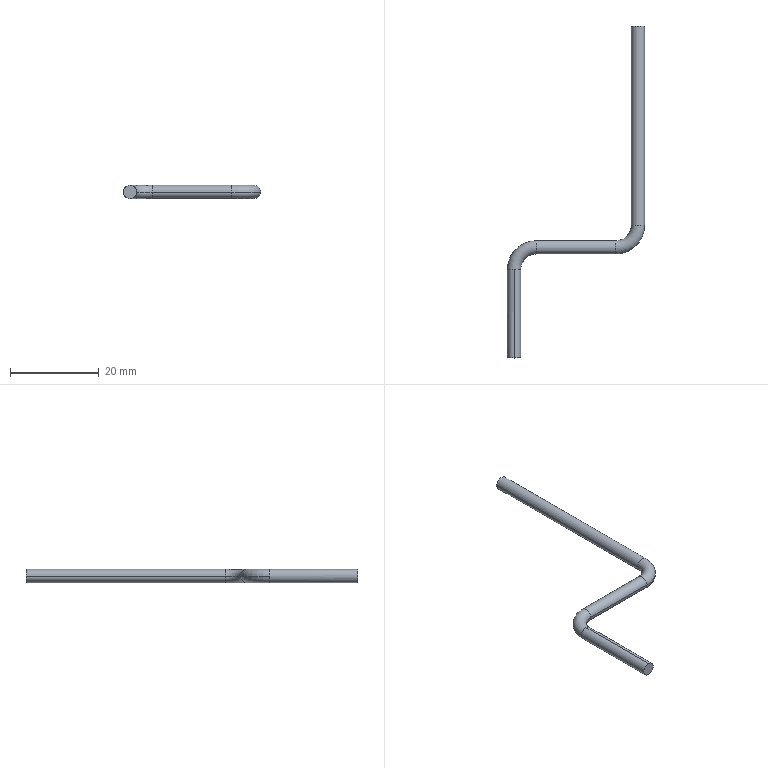Part | SolidWorks | features BaseBody 1 | 1 solid | 12 faces | box 31 x 75 x 3 mm | volume 697.725 mm3 | cylinder 6 | torus 4 | plane 2 | commonest cylinder face diameters 3 x6
STEP:
#1=CARTESIAN_POINT('',(23.,23.5,0.));
#2=VERTEX_POINT('',#1);
#3=CARTESIAN_POINT('',(23.,26.5,0.));
#4=VERTEX_POINT('',#3);
#5=CARTESIAN_POINT('',(23.,25.,0.));
#6=DIRECTION('',(-1.,0.,0.));
#7=DIRECTION('',(0.,0.,-1.));
#8=AXIS2_PLACEMENT_3D('',#5,#6,#7);
#9=CIRCLE('',#8,1.5);
#10=EDGE_CURVE('',#2,#4,#9,.T.);
#11=ORIENTED_EDGE('',*,*,#10,.F.);
#12=CARTESIAN_POINT('',(29.5,30.,0.));
#13=VERTEX_POINT('',#12);
#14=CARTESIAN_POINT('',(23.,30.,0.));
#15=DIRECTION('',(0.,0.,1.));
#16=DIRECTION('',(1.,0.,0.));
#17=AXIS2_PLACEMENT_3D('',#14,#15,#16);
#18=CIRCLE('',#17,6.5);
#19=EDGE_CURVE('',#2,#13,#18,.T.);
#20=ORIENTED_EDGE('',*,*,#19,.T.);
#21=CARTESIAN_POINT('',(26.5,30.,0.));
#22=VERTEX_POINT('',#21);
#23=CARTESIAN_POINT('',(28.,30.,0.));
#24=DIRECTION('',(0.,-1.,0.));
#25=DIRECTION('',(0.,0.,-1.));
#26=AXIS2_PLACEMENT_3D('',#23,#24,#25);
#27=CIRCLE('',#26,1.5);
#28=EDGE_CURVE('',#13,#22,#27,.T.);
#29=ORIENTED_EDGE('',*,*,#28,.T.);
#30=CARTESIAN_POINT('',(23.,30.,0.));
#31=DIRECTION('',(0.,0.,1.));
#32=DIRECTION('',(1.,0.,0.));
#33=AXIS2_PLACEMENT_3D('',#30,#31,#32);
#34=CIRCLE('',#33,3.5);
#35=EDGE_CURVE('',#4,#22,#34,.T.);
#36=ORIENTED_EDGE('',*,*,#35,.F.);
#37=EDGE_LOOP('',(#11,#20,#29,#36));
#38=FACE_OUTER_BOUND('',#37,.T.);
#39=CARTESIAN_POINT('',(23.,30.,0.));
#40=DIRECTION('',(0.,0.,1.));
#41=DIRECTION('',(1.,0.,0.));
#42=AXIS2_PLACEMENT_3D('',#39,#40,#41);
#43=TOROIDAL_SURFACE('',#42,5.,1.5);
#44=ADVANCED_FACE('',(#38),#43,.T.);
#45=CARTESIAN_POINT('',(-1.5,20.,0.));
#46=VERTEX_POINT('',#45);
#47=CARTESIAN_POINT('',(0.,20.,-1.5));
#48=VERTEX_POINT('',#47);
#49=CARTESIAN_POINT('',(0.,20.,0.));
#50=DIRECTION('',(0.,-1.,0.));
#51=DIRECTION('',(0.,0.,-1.));
#52=AXIS2_PLACEMENT_3D('',#49,#50,#51);
#53=CIRCLE('',#52,1.5);
#54=EDGE_CURVE('',#46,#48,#53,.T.);
#55=ORIENTED_EDGE('',*,*,#54,.F.);
#56=CARTESIAN_POINT('',(5.,26.5,0.));
#57=VERTEX_POINT('',#56);
#58=CARTESIAN_POINT('',(5.,20.,0.));
#59=DIRECTION('',(0.,0.,-1.));
#60=DIRECTION('',(-1.,0.,0.));
#61=AXIS2_PLACEMENT_3D('',#58,#59,#60);
#62=CIRCLE('',#61,6.5);
#63=EDGE_CURVE('',#46,#57,#62,.T.);
#64=ORIENTED_EDGE('',*,*,#63,.T.);
#65=CARTESIAN_POINT('',(5.,23.5,0.));
#66=VERTEX_POINT('',#65);
#67=CARTESIAN_POINT('',(5.,25.,0.));
#68=DIRECTION('',(-1.,0.,0.));
#69=DIRECTION('',(0.,0.,-1.));
#70=AXIS2_PLACEMENT_3D('',#67,#68,#69);
#71=CIRCLE('',#70,1.5);
#72=EDGE_CURVE('',#57,#66,#71,.T.);
#73=ORIENTED_EDGE('',*,*,#72,.T.);
#74=CARTESIAN_POINT('',(1.5,20.,0.));
#75=VERTEX_POINT('',#74);
#76=CARTESIAN_POINT('',(5.,20.,0.));
#77=DIRECTION('',(0.,0.,-1.));
#78=DIRECTION('',(-1.,0.,0.));
#79=AXIS2_PLACEMENT_3D('',#76,#77,#78);
#80=CIRCLE('',#79,3.5);
#81=EDGE_CURVE('',#75,#66,#80,.T.);
#82=ORIENTED_EDGE('',*,*,#81,.F.);
#83=CARTESIAN_POINT('',(0.,20.,0.));
#84=DIRECTION('',(0.,-1.,0.));
#85=DIRECTION('',(0.,0.,-1.));
#86=AXIS2_PLACEMENT_3D('',#83,#84,#85);
#87=CIRCLE('',#86,1.5);
#88=EDGE_CURVE('',#48,#75,#87,.T.);
#89=ORIENTED_EDGE('',*,*,#88,.F.);
#90=EDGE_LOOP('',(#55,#64,#73,#82,#89));
#91=FACE_OUTER_BOUND('',#90,.T.);
#92=CARTESIAN_POINT('',(5.,20.,0.));
#93=DIRECTION('',(0.,0.,-1.));
#94=DIRECTION('',(-1.,0.,0.));
#95=AXIS2_PLACEMENT_3D('',#92,#93,#94);
#96=TOROIDAL_SURFACE('',#95,5.,1.5);
#97=ADVANCED_FACE('',(#91),#96,.T.);
#98=ORIENTED_EDGE('',*,*,#28,.F.);
#99=CARTESIAN_POINT('',(29.5,75.,0.));
#100=VERTEX_POINT('',#99);
#101=CARTESIAN_POINT('',(29.5,30.,0.));
#102=DIRECTION('',(0.,1.,0.));
#103=VECTOR('',#102,1000.);
#104=LINE('',#101,#103);
#105=EDGE_CURVE('',#13,#100,#104,.T.);
#106=ORIENTED_EDGE('',*,*,#105,.T.);
#107=CARTESIAN_POINT('',(26.5,75.,0.));
#108=VERTEX_POINT('',#107);
#109=CARTESIAN_POINT('',(28.,75.,0.));
#110=DIRECTION('',(0.,-1.,0.));
#111=DIRECTION('',(0.,0.,-1.));
#112=AXIS2_PLACEMENT_3D('',#109,#110,#111);
#113=CIRCLE('',#112,1.5);
#114=EDGE_CURVE('',#100,#108,#113,.T.);
#115=ORIENTED_EDGE('',*,*,#114,.T.);
#116=CARTESIAN_POINT('',(26.5,30.,0.));
#117=DIRECTION('',(0.,1.,0.));
#118=VECTOR('',#117,1000.);
#119=LINE('',#116,#118);
#120=EDGE_CURVE('',#22,#108,#119,.T.);
#121=ORIENTED_EDGE('',*,*,#120,.F.);
#122=EDGE_LOOP('',(#98,#106,#115,#121));
#123=FACE_OUTER_BOUND('',#122,.T.);
#124=CARTESIAN_POINT('',(28.,30.,0.));
#125=DIRECTION('',(0.,1.,0.));
#126=DIRECTION('',(-1.,0.,0.));
#127=AXIS2_PLACEMENT_3D('',#124,#125,#126);
#128=CYLINDRICAL_SURFACE('',#127,1.5);
#129=ADVANCED_FACE('',(#123),#128,.T.);
#130=CARTESIAN_POINT('',(5.,25.,0.));
#131=DIRECTION('',(-1.,0.,0.));
#132=DIRECTION('',(0.,0.,-1.));
#133=AXIS2_PLACEMENT_3D('',#130,#131,#132);
#134=CIRCLE('',#133,1.5);
#135=EDGE_CURVE('',#66,#57,#134,.T.);
#136=ORIENTED_EDGE('',*,*,#135,.F.);
#137=CARTESIAN_POINT('',(5.,23.5,0.));
#138=DIRECTION('',(1.,0.,0.));
#139=VECTOR('',#138,1000.);
#140=LINE('',#137,#139);
#141=EDGE_CURVE('',#66,#2,#140,.T.);
#142=ORIENTED_EDGE('',*,*,#141,.T.);
#143=ORIENTED_EDGE('',*,*,#10,.T.);
#144=CARTESIAN_POINT('',(5.,26.5,0.));
#145=DIRECTION('',(1.,0.,0.));
#146=VECTOR('',#145,1000.);
#147=LINE('',#144,#146);
#148=EDGE_CURVE('',#57,#4,#147,.T.);
#149=ORIENTED_EDGE('',*,*,#148,.F.);
#150=EDGE_LOOP('',(#136,#142,#143,#149));
#151=FACE_OUTER_BOUND('',#150,.T.);
#152=CARTESIAN_POINT('',(5.,25.,0.));
#153=DIRECTION('',(1.,0.,0.));
#154=DIRECTION('',(0.,1.,0.));
#155=AXIS2_PLACEMENT_3D('',#152,#153,#154);
#156=CYLINDRICAL_SURFACE('',#155,1.5);
#157=ADVANCED_FACE('',(#151),#156,.T.);
#158=CARTESIAN_POINT('',(0.,0.,-1.5));
#159=VERTEX_POINT('',#158);
#160=CARTESIAN_POINT('',(0.,0.,1.5));
#161=VERTEX_POINT('',#160);
#162=CARTESIAN_POINT('',(0.,0.,0.));
#163=DIRECTION('',(0.,-1.,0.));
#164=DIRECTION('',(0.,0.,-1.));
#165=AXIS2_PLACEMENT_3D('',#162,#163,#164);
#166=CIRCLE('',#165,1.5);
#167=EDGE_CURVE('',#159,#161,#166,.T.);
#168=ORIENTED_EDGE('',*,*,#167,.F.);
#169=CARTESIAN_POINT('',(0.,0.,-1.5));
#170=DIRECTION('',(0.,1.,0.));
#171=VECTOR('',#170,1000.);
#172=LINE('',#169,#171);
#173=EDGE_CURVE('',#159,#48,#172,.T.);
#174=ORIENTED_EDGE('',*,*,#173,.T.);
#175=ORIENTED_EDGE('',*,*,#88,.T.);
#176=CARTESIAN_POINT('',(0.,20.,1.5));
#177=VERTEX_POINT('',#176);
#178=CARTESIAN_POINT('',(0.,20.,0.));
#179=DIRECTION('',(0.,-1.,0.));
#180=DIRECTION('',(0.,0.,-1.));
#181=AXIS2_PLACEMENT_3D('',#178,#179,#180);
#182=CIRCLE('',#181,1.5);
#183=EDGE_CURVE('',#75,#177,#182,.T.);
#184=ORIENTED_EDGE('',*,*,#183,.T.);
#185=CARTESIAN_POINT('',(0.,0.,1.5));
#186=DIRECTION('',(0.,1.,0.));
#187=VECTOR('',#186,1000.);
#188=LINE('',#185,#187);
#189=EDGE_CURVE('',#161,#177,#188,.T.);
#190=ORIENTED_EDGE('',*,*,#189,.F.);
#191=EDGE_LOOP('',(#168,#174,#175,#184,#190));
#192=FACE_OUTER_BOUND('',#191,.T.);
#193=CARTESIAN_POINT('',(0.,0.,0.));
#194=DIRECTION('',(0.,1.,0.));
#195=DIRECTION('',(0.,0.,1.));
#196=AXIS2_PLACEMENT_3D('',#193,#194,#195);
#197=CYLINDRICAL_SURFACE('',#196,1.5);
#198=ADVANCED_FACE('',(#192),#197,.T.);
#199=CARTESIAN_POINT('',(0.,0.,0.));
#200=DIRECTION('',(0.,-1.,0.));
#201=DIRECTION('',(0.,0.,-1.));
#202=AXIS2_PLACEMENT_3D('',#199,#200,#201);
#203=CIRCLE('',#202,1.5);
#204=EDGE_CURVE('',#161,#159,#203,.T.);
#205=ORIENTED_EDGE('',*,*,#204,.T.);
#206=ORIENTED_EDGE('',*,*,#167,.T.);
#207=EDGE_LOOP('',(#205,#206));
#208=FACE_OUTER_BOUND('',#207,.T.);
#209=CARTESIAN_POINT('',(0.,0.,0.));
#210=DIRECTION('',(0.,-1.,0.));
#211=DIRECTION('',(0.,0.,-1.));
#212=AXIS2_PLACEMENT_3D('',#209,#210,#211);
#213=PLANE('',#212);
#214=ADVANCED_FACE('',(#208),#213,.T.);
#215=CARTESIAN_POINT('',(28.,75.,0.));
#216=DIRECTION('',(0.,-1.,0.));
#217=DIRECTION('',(0.,0.,-1.));
#218=AXIS2_PLACEMENT_3D('',#215,#216,#217);
#219=CIRCLE('',#218,1.5);
#220=EDGE_CURVE('',#108,#100,#219,.T.);
#221=ORIENTED_EDGE('',*,*,#220,.F.);
#222=ORIENTED_EDGE('',*,*,#114,.F.);
#223=EDGE_LOOP('',(#221,#222));
#224=FACE_OUTER_BOUND('',#223,.T.);
#225=CARTESIAN_POINT('',(28.,75.,0.));
#226=DIRECTION('',(0.,-1.,0.));
#227=DIRECTION('',(0.,0.,-1.));
#228=AXIS2_PLACEMENT_3D('',#225,#226,#227);
#229=PLANE('',#228);
#230=ADVANCED_FACE('',(#224),#229,.F.);
#231=ORIENTED_EDGE('',*,*,#173,.F.);
#232=ORIENTED_EDGE('',*,*,#204,.F.);
#233=ORIENTED_EDGE('',*,*,#189,.T.);
#234=CARTESIAN_POINT('',(0.,20.,0.));
#235=DIRECTION('',(0.,-1.,0.));
#236=DIRECTION('',(0.,0.,-1.));
#237=AXIS2_PLACEMENT_3D('',#234,#235,#236);
#238=CIRCLE('',#237,1.5);
#239=EDGE_CURVE('',#177,#46,#238,.T.);
#240=ORIENTED_EDGE('',*,*,#239,.T.);
#241=ORIENTED_EDGE('',*,*,#54,.T.);
#242=EDGE_LOOP('',(#231,#232,#233,#240,#241));
#243=FACE_OUTER_BOUND('',#242,.T.);
#244=CARTESIAN_POINT('',(0.,0.,0.));
#245=DIRECTION('',(0.,1.,0.));
#246=DIRECTION('',(0.,0.,1.));
#247=AXIS2_PLACEMENT_3D('',#244,#245,#246);
#248=CYLINDRICAL_SURFACE('',#247,1.5);
#249=ADVANCED_FACE('',(#243),#248,.T.);
#250=ORIENTED_EDGE('',*,*,#63,.F.);
#251=ORIENTED_EDGE('',*,*,#239,.F.);
#252=ORIENTED_EDGE('',*,*,#183,.F.);
#253=ORIENTED_EDGE('',*,*,#81,.T.);
#254=ORIENTED_EDGE('',*,*,#135,.T.);
#255=EDGE_LOOP('',(#250,#251,#252,#253,#254));
#256=FACE_OUTER_BOUND('',#255,.T.);
#257=CARTESIAN_POINT('',(5.,20.,0.));
#258=DIRECTION('',(0.,0.,-1.));
#259=DIRECTION('',(-1.,0.,0.));
#260=AXIS2_PLACEMENT_3D('',#257,#258,#259);
#261=TOROIDAL_SURFACE('',#260,5.,1.5);
#262=ADVANCED_FACE('',(#256),#261,.T.);
#263=ORIENTED_EDGE('',*,*,#141,.F.);
#264=ORIENTED_EDGE('',*,*,#72,.F.);
#265=ORIENTED_EDGE('',*,*,#148,.T.);
#266=CARTESIAN_POINT('',(23.,25.,0.));
#267=DIRECTION('',(-1.,0.,0.));
#268=DIRECTION('',(0.,0.,-1.));
#269=AXIS2_PLACEMENT_3D('',#266,#267,#268);
#270=CIRCLE('',#269,1.5);
#271=EDGE_CURVE('',#4,#2,#270,.T.);
#272=ORIENTED_EDGE('',*,*,#271,.T.);
#273=EDGE_LOOP('',(#263,#264,#265,#272));
#274=FACE_OUTER_BOUND('',#273,.T.);
#275=CARTESIAN_POINT('',(5.,25.,0.));
#276=DIRECTION('',(1.,0.,0.));
#277=DIRECTION('',(0.,1.,0.));
#278=AXIS2_PLACEMENT_3D('',#275,#276,#277);
#279=CYLINDRICAL_SURFACE('',#278,1.5);
#280=ADVANCED_FACE('',(#274),#279,.T.);
#281=ORIENTED_EDGE('',*,*,#19,.F.);
#282=ORIENTED_EDGE('',*,*,#271,.F.);
#283=ORIENTED_EDGE('',*,*,#35,.T.);
#284=CARTESIAN_POINT('',(28.,30.,0.));
#285=DIRECTION('',(0.,-1.,0.));
#286=DIRECTION('',(0.,0.,-1.));
#287=AXIS2_PLACEMENT_3D('',#284,#285,#286);
#288=CIRCLE('',#287,1.5);
#289=EDGE_CURVE('',#22,#13,#288,.T.);
#290=ORIENTED_EDGE('',*,*,#289,.T.);
#291=EDGE_LOOP('',(#281,#282,#283,#290));
#292=FACE_OUTER_BOUND('',#291,.T.);
#293=CARTESIAN_POINT('',(23.,30.,0.));
#294=DIRECTION('',(0.,0.,1.));
#295=DIRECTION('',(1.,0.,0.));
#296=AXIS2_PLACEMENT_3D('',#293,#294,#295);
#297=TOROIDAL_SURFACE('',#296,5.,1.5);
#298=ADVANCED_FACE('',(#292),#297,.T.);
#299=ORIENTED_EDGE('',*,*,#105,.F.);
#300=ORIENTED_EDGE('',*,*,#289,.F.);
#301=ORIENTED_EDGE('',*,*,#120,.T.);
#302=ORIENTED_EDGE('',*,*,#220,.T.);
#303=EDGE_LOOP('',(#299,#300,#301,#302));
#304=FACE_OUTER_BOUND('',#303,.T.);
#305=CARTESIAN_POINT('',(28.,30.,0.));
#306=DIRECTION('',(0.,1.,0.));
#307=DIRECTION('',(-1.,0.,0.));
#308=AXIS2_PLACEMENT_3D('',#305,#306,#307);
#309=CYLINDRICAL_SURFACE('',#308,1.5);
#310=ADVANCED_FACE('',(#304),#309,.T.);
#311=CLOSED_SHELL('',(#44,#97,#129,#157,#198,#214,#230,#249,#262,#280,#298,#310));
#312=MANIFOLD_SOLID_BREP('',#311);
#313=CARTESIAN_POINT('',(0.,0.,0.));
#314=DIRECTION('',(0.,0.,1.));
#315=DIRECTION('',(1.,0.,0.));
#316=AXIS2_PLACEMENT_3D('',#313,#314,#315);
#317=(LENGTH_UNIT()NAMED_UNIT(*)SI_UNIT(.MILLI.,.METRE.));
#318=UNCERTAINTY_MEASURE_WITH_UNIT(LENGTH_MEASURE(0.00001),#317,'','');
#319=(NAMED_UNIT(*)PLANE_ANGLE_UNIT()SI_UNIT($,.RADIAN.));
#320=(NAMED_UNIT(*)SI_UNIT($,.STERADIAN.)SOLID_ANGLE_UNIT());
#321=(GEOMETRIC_REPRESENTATION_CONTEXT(3)GLOBAL_UNCERTAINTY_ASSIGNED_CONTEXT((#318))GLOBAL_UNIT_ASSIGNED_CONTEXT((#317,#319,#320))REPRESENTATION_CONTEXT('',''));
#322=ADVANCED_BREP_SHAPE_REPRESENTATION('',(#312,#316),#321);